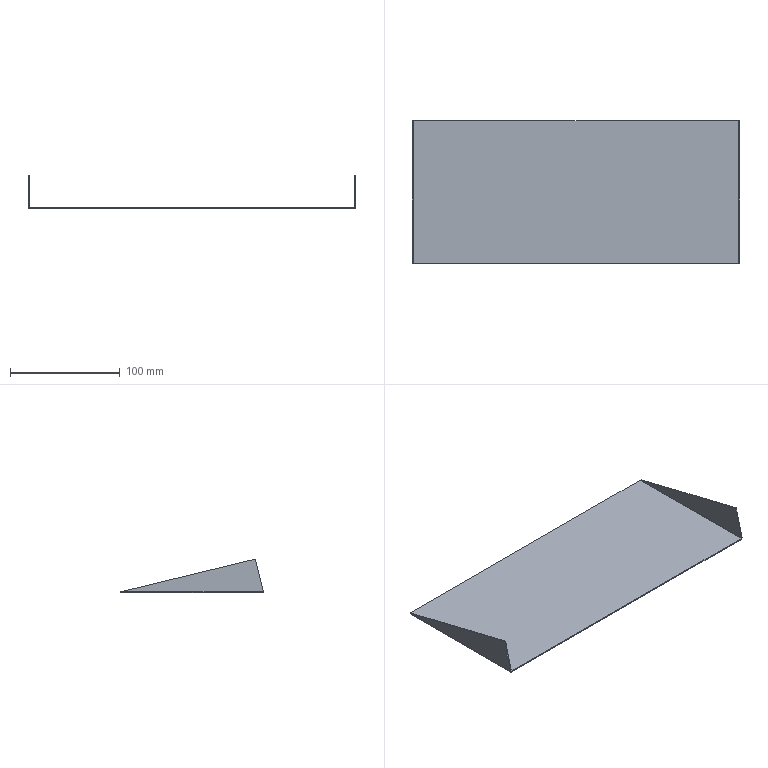Part | SolidWorks | features EdgeFlange 1, FlatPattern 1, MirrorPattern 1, SMBaseFlange 1, SheetMetal 1 | 1 solid | 20 faces | box 299 x 130.5 x 31 mm | volume 42855 mm3 | plane 12 | spline 4 | cylinder 4 | commonest cylinder face diameters 0.4 x2 2.4 x2
STEP:
#1=CARTESIAN_POINT('',(148.3,65.25,-1.));
#2=VERTEX_POINT('',#1);
#3=CARTESIAN_POINT('',(148.3,-65.25,-1.));
#4=VERTEX_POINT('',#3);
#5=CARTESIAN_POINT('',(148.3,65.25,-1.));
#6=DIRECTION('',(0.,-1.,0.));
#7=VECTOR('',#6,1000.);
#8=LINE('',#5,#7);
#9=EDGE_CURVE('',#2,#4,#8,.T.);
#10=ORIENTED_EDGE('',*,*,#9,.T.);
#11=CARTESIAN_POINT('',(-148.3,-65.25,-1.));
#12=VERTEX_POINT('',#11);
#13=CARTESIAN_POINT('',(-149.5,-65.25,-1.));
#14=DIRECTION('',(1.,0.,0.));
#15=VECTOR('',#14,1000.);
#16=LINE('',#13,#15);
#17=EDGE_CURVE('',#12,#4,#16,.T.);
#18=ORIENTED_EDGE('',*,*,#17,.F.);
#19=CARTESIAN_POINT('',(-148.3,65.25,-1.));
#20=VERTEX_POINT('',#19);
#21=CARTESIAN_POINT('',(-148.3,-65.25,-1.));
#22=DIRECTION('',(0.,1.,0.));
#23=VECTOR('',#22,1000.);
#24=LINE('',#21,#23);
#25=EDGE_CURVE('',#12,#20,#24,.T.);
#26=ORIENTED_EDGE('',*,*,#25,.T.);
#27=CARTESIAN_POINT('',(-149.5,65.25,-1.));
#28=DIRECTION('',(-1.,0.,0.));
#29=VECTOR('',#28,1000.);
#30=LINE('',#27,#29);
#31=EDGE_CURVE('',#2,#20,#30,.T.);
#32=ORIENTED_EDGE('',*,*,#31,.F.);
#33=EDGE_LOOP('',(#10,#18,#26,#32));
#34=FACE_OUTER_BOUND('',#33,.T.);
#35=CARTESIAN_POINT('',(0.,0.,-1.));
#36=DIRECTION('',(0.,0.,1.));
#37=DIRECTION('',(1.,0.,0.));
#38=AXIS2_PLACEMENT_3D('',#35,#36,#37);
#39=PLANE('',#38);
#40=ADVANCED_FACE('',(#34),#39,.F.);
#41=CARTESIAN_POINT('',(-148.3,-65.25,0.));
#42=VERTEX_POINT('',#41);
#43=CARTESIAN_POINT('',(148.3,-65.25,0.));
#44=VERTEX_POINT('',#43);
#45=CARTESIAN_POINT('',(-149.5,-65.25,0.));
#46=DIRECTION('',(1.,0.,0.));
#47=VECTOR('',#46,1000.);
#48=LINE('',#45,#47);
#49=EDGE_CURVE('',#42,#44,#48,.T.);
#50=ORIENTED_EDGE('',*,*,#49,.T.);
#51=CARTESIAN_POINT('',(148.3,65.25,0.));
#52=VERTEX_POINT('',#51);
#53=CARTESIAN_POINT('',(148.3,65.25,0.));
#54=DIRECTION('',(0.,-1.,0.));
#55=VECTOR('',#54,1000.);
#56=LINE('',#53,#55);
#57=EDGE_CURVE('',#52,#44,#56,.T.);
#58=ORIENTED_EDGE('',*,*,#57,.F.);
#59=CARTESIAN_POINT('',(-148.3,65.25,0.));
#60=VERTEX_POINT('',#59);
#61=CARTESIAN_POINT('',(-149.5,65.25,0.));
#62=DIRECTION('',(-1.,0.,0.));
#63=VECTOR('',#62,1000.);
#64=LINE('',#61,#63);
#65=EDGE_CURVE('',#52,#60,#64,.T.);
#66=ORIENTED_EDGE('',*,*,#65,.T.);
#67=CARTESIAN_POINT('',(-148.3,-65.25,0.));
#68=DIRECTION('',(0.,1.,0.));
#69=VECTOR('',#68,1000.);
#70=LINE('',#67,#69);
#71=EDGE_CURVE('',#42,#60,#70,.T.);
#72=ORIENTED_EDGE('',*,*,#71,.F.);
#73=EDGE_LOOP('',(#50,#58,#66,#72));
#74=FACE_OUTER_BOUND('',#73,.T.);
#75=CARTESIAN_POINT('',(0.,0.,0.));
#76=DIRECTION('',(0.,0.,1.));
#77=DIRECTION('',(1.,0.,0.));
#78=AXIS2_PLACEMENT_3D('',#75,#76,#77);
#79=PLANE('',#78);
#80=ADVANCED_FACE('',(#74),#79,.T.);
#81=ORIENTED_EDGE('',*,*,#65,.F.);
#82=CARTESIAN_POINT('',(148.3,65.25,0.));
#83=DIRECTION('',(0.,0.,-1.));
#84=VECTOR('',#83,1000.);
#85=LINE('',#82,#84);
#86=EDGE_CURVE('',#52,#2,#85,.T.);
#87=ORIENTED_EDGE('',*,*,#86,.T.);
#88=ORIENTED_EDGE('',*,*,#31,.T.);
#89=CARTESIAN_POINT('',(-148.3,65.25,0.));
#90=DIRECTION('',(0.,0.,-1.));
#91=VECTOR('',#90,1000.);
#92=LINE('',#89,#91);
#93=EDGE_CURVE('',#60,#20,#92,.T.);
#94=ORIENTED_EDGE('',*,*,#93,.F.);
#95=EDGE_LOOP('',(#81,#87,#88,#94));
#96=FACE_OUTER_BOUND('',#95,.T.);
#97=CARTESIAN_POINT('',(-149.5,65.25,-1.));
#98=DIRECTION('',(0.,1.,0.));
#99=DIRECTION('',(0.,0.,1.));
#100=AXIS2_PLACEMENT_3D('',#97,#98,#99);
#101=PLANE('',#100);
#102=ADVANCED_FACE('',(#96),#101,.T.);
#103=CARTESIAN_POINT('',(148.3,-65.25,0.));
#104=DIRECTION('',(0.,0.,-1.));
#105=VECTOR('',#104,1000.);
#106=LINE('',#103,#105);
#107=EDGE_CURVE('',#44,#4,#106,.T.);
#108=ORIENTED_EDGE('',*,*,#107,.F.);
#109=ORIENTED_EDGE('',*,*,#49,.F.);
#110=CARTESIAN_POINT('',(-148.3,-65.25,0.));
#111=DIRECTION('',(0.,0.,-1.));
#112=VECTOR('',#111,1000.);
#113=LINE('',#110,#112);
#114=EDGE_CURVE('',#42,#12,#113,.T.);
#115=ORIENTED_EDGE('',*,*,#114,.T.);
#116=ORIENTED_EDGE('',*,*,#17,.T.);
#117=EDGE_LOOP('',(#108,#109,#115,#116));
#118=FACE_OUTER_BOUND('',#117,.T.);
#119=CARTESIAN_POINT('',(-149.5,-65.25,-1.));
#120=DIRECTION('',(0.,-1.,0.));
#121=DIRECTION('',(0.,0.,-1.));
#122=AXIS2_PLACEMENT_3D('',#119,#120,#121);
#123=PLANE('',#122);
#124=ADVANCED_FACE('',(#118),#123,.T.);
#125=CARTESIAN_POINT('',(-148.5,64.429,0.2));
#126=VERTEX_POINT('',#125);
#127=CARTESIAN_POINT('',(-149.5,64.429,0.2));
#128=VERTEX_POINT('',#127);
#129=CARTESIAN_POINT('',(-149.5,64.429,0.2));
#130=DIRECTION('',(-1.,0.,0.));
#131=VECTOR('',#130,1000.);
#132=LINE('',#129,#131);
#133=EDGE_CURVE('',#126,#128,#132,.T.);
#134=ORIENTED_EDGE('',*,*,#133,.F.);
#135=CARTESIAN_POINT('',(-148.3,65.25,0.));
#136=CARTESIAN_POINT('',(-148.352,65.113,0.));
#137=CARTESIAN_POINT('',(-148.404,64.976,0.02155));
#138=CARTESIAN_POINT('',(-148.478,64.702,0.0956));
#139=CARTESIAN_POINT('',(-148.5,64.566,0.1476));
#140=CARTESIAN_POINT('',(-148.5,64.429,0.2));
#141=B_SPLINE_CURVE_WITH_KNOTS('',3,(#135,#136,#137,#138,#139,#140),.UNSPECIFIED.,.F.,.F.,(4,2,4),(0.,0.5,1.),.UNSPECIFIED.);
#142=EDGE_CURVE('',#60,#126,#141,.T.);
#143=ORIENTED_EDGE('',*,*,#142,.F.);
#144=ORIENTED_EDGE('',*,*,#93,.T.);
#145=CARTESIAN_POINT('',(-148.3,65.25,-1.));
#146=CARTESIAN_POINT('',(-148.459,65.181,-1.));
#147=CARTESIAN_POINT('',(-148.612,65.114,-0.9695));
#148=CARTESIAN_POINT('',(-148.905,64.976,-0.8483));
#149=CARTESIAN_POINT('',(-149.036,64.908,-0.7606));
#150=CARTESIAN_POINT('',(-149.26,64.771,-0.5372));
#151=CARTESIAN_POINT('',(-149.348,64.703,-0.4051));
#152=CARTESIAN_POINT('',(-149.469,64.566,-0.1141));
#153=CARTESIAN_POINT('',(-149.5,64.498,0.04143));
#154=CARTESIAN_POINT('',(-149.5,64.429,0.2));
#155=B_SPLINE_CURVE_WITH_KNOTS('',3,(#145,#146,#147,#148,#149,#150,#151,#152,#153,#154),.UNSPECIFIED.,.F.,.F.,(4,2,2,2,4),(0.,0.0005105,0.001021,0.001532,0.002042),.UNSPECIFIED.);
#156=EDGE_CURVE('',#20,#128,#155,.T.);
#157=ORIENTED_EDGE('',*,*,#156,.T.);
#158=EDGE_LOOP('',(#134,#143,#144,#157));
#159=FACE_OUTER_BOUND('',#158,.T.);
#160=CARTESIAN_POINT('',(-148.3,65.25,-1.01));
#161=CARTESIAN_POINT('',(-148.458,65.182,-1.01));
#162=CARTESIAN_POINT('',(-148.617,65.113,-0.9785));
#163=CARTESIAN_POINT('',(-148.909,64.976,-0.8573));
#164=CARTESIAN_POINT('',(-149.044,64.908,-0.7676));
#165=CARTESIAN_POINT('',(-149.268,64.771,-0.5436));
#166=CARTESIAN_POINT('',(-149.357,64.702,-0.4094));
#167=CARTESIAN_POINT('',(-149.479,64.566,-0.1167));
#168=CARTESIAN_POINT('',(-149.51,64.497,0.04159));
#169=CARTESIAN_POINT('',(-149.51,64.429,0.2));
#170=CARTESIAN_POINT('',(-148.3,65.25,-1.));
#171=CARTESIAN_POINT('',(-148.457,65.182,-1.));
#172=CARTESIAN_POINT('',(-148.614,65.113,-0.9688));
#173=CARTESIAN_POINT('',(-148.904,64.976,-0.8485));
#174=CARTESIAN_POINT('',(-149.037,64.908,-0.7596));
#175=CARTESIAN_POINT('',(-149.26,64.771,-0.5375));
#176=CARTESIAN_POINT('',(-149.349,64.702,-0.4043));
#177=CARTESIAN_POINT('',(-149.469,64.566,-0.1141));
#178=CARTESIAN_POINT('',(-149.5,64.497,0.0429));
#179=CARTESIAN_POINT('',(-149.5,64.429,0.2));
#180=CARTESIAN_POINT('',(-148.3,65.25,0.));
#181=CARTESIAN_POINT('',(-148.326,65.182,0.));
#182=CARTESIAN_POINT('',(-148.352,65.113,0.005205));
#183=CARTESIAN_POINT('',(-148.401,64.976,0.02524));
#184=CARTESIAN_POINT('',(-148.423,64.908,0.04007));
#185=CARTESIAN_POINT('',(-148.46,64.771,0.07709));
#186=CARTESIAN_POINT('',(-148.475,64.702,0.09928));
#187=CARTESIAN_POINT('',(-148.495,64.566,0.1477));
#188=CARTESIAN_POINT('',(-148.5,64.497,0.1738));
#189=CARTESIAN_POINT('',(-148.5,64.429,0.2));
#190=CARTESIAN_POINT('',(-148.3,65.25,0.0101));
#191=CARTESIAN_POINT('',(-148.325,65.182,0.0101));
#192=CARTESIAN_POINT('',(-148.35,65.113,0.01504));
#193=CARTESIAN_POINT('',(-148.396,64.976,0.03407));
#194=CARTESIAN_POINT('',(-148.417,64.908,0.04814));
#195=CARTESIAN_POINT('',(-148.452,64.771,0.0833));
#196=CARTESIAN_POINT('',(-148.466,64.702,0.1044));
#197=CARTESIAN_POINT('',(-148.485,64.566,0.1503));
#198=CARTESIAN_POINT('',(-148.49,64.497,0.1751));
#199=CARTESIAN_POINT('',(-148.49,64.429,0.2));
#200=B_SPLINE_SURFACE_WITH_KNOTS('',1,3,((#160,#161,#162,#163,#164,#165,#166,#167,#168,#169),(#170,#171,#172,#173,#174,#175,#176,#177,#178,#179),(#180,#181,#182,#183,#184,#185,#186,#187,#188,#189),(#190,#191,#192,#193,#194,#195,#196,#197,#198,#199)),.UNSPECIFIED.,.F.,.F.,.F.,(2,1,1,2),(4,2,2,2,4),(-0.01,0.,1.,1.01),(0.,0.25,0.5,0.75,1.),.UNSPECIFIED.);
#201=ADVANCED_FACE('',(#159),#200,.F.);
#202=CARTESIAN_POINT('',(-148.5,-65.201,0.2));
#203=VERTEX_POINT('',#202);
#204=CARTESIAN_POINT('',(-148.5,-65.201,0.2));
#205=CARTESIAN_POINT('',(-148.5,-65.209,0.1476));
#206=CARTESIAN_POINT('',(-148.478,-65.218,0.0956));
#207=CARTESIAN_POINT('',(-148.404,-65.234,0.02155));
#208=CARTESIAN_POINT('',(-148.352,-65.242,0.));
#209=CARTESIAN_POINT('',(-148.3,-65.25,0.));
#210=B_SPLINE_CURVE_WITH_KNOTS('',3,(#204,#205,#206,#207,#208,#209),.UNSPECIFIED.,.F.,.F.,(4,2,4),(0.,0.5,1.),.UNSPECIFIED.);
#211=EDGE_CURVE('',#203,#42,#210,.T.);
#212=ORIENTED_EDGE('',*,*,#211,.F.);
#213=CARTESIAN_POINT('',(-149.5,-65.201,0.2));
#214=VERTEX_POINT('',#213);
#215=CARTESIAN_POINT('',(-148.5,-65.201,0.2));
#216=DIRECTION('',(-1.,0.,0.));
#217=VECTOR('',#216,1000.);
#218=LINE('',#215,#217);
#219=EDGE_CURVE('',#203,#214,#218,.T.);
#220=ORIENTED_EDGE('',*,*,#219,.T.);
#221=CARTESIAN_POINT('',(-149.5,-65.201,0.2));
#222=CARTESIAN_POINT('',(-149.5,-65.205,0.04292));
#223=CARTESIAN_POINT('',(-149.469,-65.209,-0.1141));
#224=CARTESIAN_POINT('',(-149.349,-65.218,-0.4043));
#225=CARTESIAN_POINT('',(-149.26,-65.222,-0.5375));
#226=CARTESIAN_POINT('',(-149.037,-65.23,-0.7596));
#227=CARTESIAN_POINT('',(-148.904,-65.234,-0.8485));
#228=CARTESIAN_POINT('',(-148.614,-65.242,-0.9688));
#229=CARTESIAN_POINT('',(-148.457,-65.246,-1.));
#230=CARTESIAN_POINT('',(-148.3,-65.25,-1.));
#231=B_SPLINE_CURVE_WITH_KNOTS('',3,(#221,#222,#223,#224,#225,#226,#227,#228,#229,#230),.UNSPECIFIED.,.F.,.F.,(4,2,2,2,4),(0.,0.25,0.5,0.75,1.),.UNSPECIFIED.);
#232=EDGE_CURVE('',#214,#12,#231,.T.);
#233=ORIENTED_EDGE('',*,*,#232,.T.);
#234=ORIENTED_EDGE('',*,*,#114,.F.);
#235=EDGE_LOOP('',(#212,#220,#233,#234));
#236=FACE_OUTER_BOUND('',#235,.T.);
#237=CARTESIAN_POINT('',(-149.51,-65.201,0.2));
#238=CARTESIAN_POINT('',(-149.51,-65.205,0.04158));
#239=CARTESIAN_POINT('',(-149.479,-65.209,-0.1167));
#240=CARTESIAN_POINT('',(-149.357,-65.218,-0.4094));
#241=CARTESIAN_POINT('',(-149.268,-65.222,-0.5436));
#242=CARTESIAN_POINT('',(-149.044,-65.23,-0.7676));
#243=CARTESIAN_POINT('',(-148.909,-65.234,-0.8573));
#244=CARTESIAN_POINT('',(-148.617,-65.242,-0.9785));
#245=CARTESIAN_POINT('',(-148.458,-65.246,-1.01));
#246=CARTESIAN_POINT('',(-148.3,-65.25,-1.01));
#247=CARTESIAN_POINT('',(-149.5,-65.201,0.2));
#248=CARTESIAN_POINT('',(-149.5,-65.205,0.04289));
#249=CARTESIAN_POINT('',(-149.469,-65.209,-0.1141));
#250=CARTESIAN_POINT('',(-149.349,-65.218,-0.4043));
#251=CARTESIAN_POINT('',(-149.26,-65.222,-0.5375));
#252=CARTESIAN_POINT('',(-149.037,-65.23,-0.7596));
#253=CARTESIAN_POINT('',(-148.904,-65.234,-0.8485));
#254=CARTESIAN_POINT('',(-148.614,-65.242,-0.9688));
#255=CARTESIAN_POINT('',(-148.457,-65.246,-1.));
#256=CARTESIAN_POINT('',(-148.3,-65.25,-1.));
#257=CARTESIAN_POINT('',(-148.5,-65.201,0.2));
#258=CARTESIAN_POINT('',(-148.5,-65.205,0.1738));
#259=CARTESIAN_POINT('',(-148.495,-65.209,0.1477));
#260=CARTESIAN_POINT('',(-148.475,-65.218,0.09928));
#261=CARTESIAN_POINT('',(-148.46,-65.222,0.07709));
#262=CARTESIAN_POINT('',(-148.423,-65.23,0.04007));
#263=CARTESIAN_POINT('',(-148.401,-65.234,0.02524));
#264=CARTESIAN_POINT('',(-148.352,-65.242,0.005205));
#265=CARTESIAN_POINT('',(-148.326,-65.246,0.));
#266=CARTESIAN_POINT('',(-148.3,-65.25,0.));
#267=CARTESIAN_POINT('',(-148.49,-65.201,0.2));
#268=CARTESIAN_POINT('',(-148.49,-65.205,0.1751));
#269=CARTESIAN_POINT('',(-148.485,-65.209,0.1503));
#270=CARTESIAN_POINT('',(-148.466,-65.218,0.1044));
#271=CARTESIAN_POINT('',(-148.452,-65.222,0.0833));
#272=CARTESIAN_POINT('',(-148.417,-65.23,0.04814));
#273=CARTESIAN_POINT('',(-148.396,-65.234,0.03407));
#274=CARTESIAN_POINT('',(-148.35,-65.242,0.01504));
#275=CARTESIAN_POINT('',(-148.325,-65.246,0.0101));
#276=CARTESIAN_POINT('',(-148.3,-65.25,0.0101));
#277=B_SPLINE_SURFACE_WITH_KNOTS('',1,3,((#237,#238,#239,#240,#241,#242,#243,#244,#245,#246),(#247,#248,#249,#250,#251,#252,#253,#254,#255,#256),(#257,#258,#259,#260,#261,#262,#263,#264,#265,#266),(#267,#268,#269,#270,#271,#272,#273,#274,#275,#276)),.UNSPECIFIED.,.F.,.F.,.F.,(2,1,1,2),(4,2,2,2,4),(-0.01,0.,1.,1.01),(0.,0.25,0.5,0.75,1.),.UNSPECIFIED.);
#278=ADVANCED_FACE('',(#236),#277,.F.);
#279=ORIENTED_EDGE('',*,*,#25,.F.);
#280=ORIENTED_EDGE('',*,*,#232,.F.);
#281=CARTESIAN_POINT('',(-149.5,64.429,0.2));
#282=DIRECTION('',(0.,1.,0.));
#283=VECTOR('',#282,1000.);
#284=LINE('',#281,#283);
#285=EDGE_CURVE('',#214,#128,#284,.T.);
#286=ORIENTED_EDGE('',*,*,#285,.T.);
#287=ORIENTED_EDGE('',*,*,#156,.F.);
#288=EDGE_LOOP('',(#279,#280,#286,#287));
#289=FACE_OUTER_BOUND('',#288,.T.);
#290=CARTESIAN_POINT('',(-148.3,-65.25,0.2));
#291=DIRECTION('',(0.,-1.,0.));
#292=DIRECTION('',(-1.,0.,0.));
#293=AXIS2_PLACEMENT_3D('',#290,#291,#292);
#294=CYLINDRICAL_SURFACE('',#293,1.2);
#295=ADVANCED_FACE('',(#289),#294,.T.);
#296=ORIENTED_EDGE('',*,*,#71,.T.);
#297=ORIENTED_EDGE('',*,*,#142,.T.);
#298=CARTESIAN_POINT('',(-148.5,64.429,0.2));
#299=DIRECTION('',(0.,-1.,0.));
#300=VECTOR('',#299,1000.);
#301=LINE('',#298,#300);
#302=EDGE_CURVE('',#126,#203,#301,.T.);
#303=ORIENTED_EDGE('',*,*,#302,.T.);
#304=ORIENTED_EDGE('',*,*,#211,.T.);
#305=EDGE_LOOP('',(#296,#297,#303,#304));
#306=FACE_OUTER_BOUND('',#305,.T.);
#307=CARTESIAN_POINT('',(-148.3,-65.25,0.2));
#308=DIRECTION('',(0.,-1.,0.));
#309=DIRECTION('',(-1.,0.,0.));
#310=AXIS2_PLACEMENT_3D('',#307,#308,#309);
#311=CYLINDRICAL_SURFACE('',#310,0.2);
#312=ADVANCED_FACE('',(#306),#311,.F.);
#313=ORIENTED_EDGE('',*,*,#133,.T.);
#314=CARTESIAN_POINT('',(-149.5,-57.944,30.));
#315=VERTEX_POINT('',#314);
#316=CARTESIAN_POINT('',(-149.5,3.653,15.));
#317=DIRECTION('',(0.,0.9716,-0.2366));
#318=VECTOR('',#317,1000.);
#319=LINE('',#316,#318);
#320=EDGE_CURVE('',#315,#128,#319,.T.);
#321=ORIENTED_EDGE('',*,*,#320,.F.);
#322=CARTESIAN_POINT('',(-148.5,-57.944,30.));
#323=VERTEX_POINT('',#322);
#324=CARTESIAN_POINT('',(-149.5,-57.944,30.));
#325=DIRECTION('',(1.,0.,0.));
#326=VECTOR('',#325,1000.);
#327=LINE('',#324,#326);
#328=EDGE_CURVE('',#315,#323,#327,.T.);
#329=ORIENTED_EDGE('',*,*,#328,.T.);
#330=CARTESIAN_POINT('',(-148.5,-57.944,30.));
#331=DIRECTION('',(0.,0.9716,-0.2366));
#332=VECTOR('',#331,1000.);
#333=LINE('',#330,#332);
#334=EDGE_CURVE('',#323,#126,#333,.T.);
#335=ORIENTED_EDGE('',*,*,#334,.T.);
#336=EDGE_LOOP('',(#313,#321,#329,#335));
#337=FACE_OUTER_BOUND('',#336,.T.);
#338=CARTESIAN_POINT('',(-149.5,-57.944,30.));
#339=DIRECTION('',(0.,-0.2366,-0.9716));
#340=DIRECTION('',(0.,0.9716,-0.2366));
#341=AXIS2_PLACEMENT_3D('',#338,#339,#340);
#342=PLANE('',#341);
#343=ADVANCED_FACE('',(#337),#342,.F.);
#344=ORIENTED_EDGE('',*,*,#219,.F.);
#345=CARTESIAN_POINT('',(-148.5,-65.25,0.));
#346=DIRECTION('',(0.,0.2366,0.9716));
#347=VECTOR('',#346,1000.);
#348=LINE('',#345,#347);
#349=EDGE_CURVE('',#203,#323,#348,.T.);
#350=ORIENTED_EDGE('',*,*,#349,.T.);
#351=ORIENTED_EDGE('',*,*,#328,.F.);
#352=CARTESIAN_POINT('',(-149.5,-61.597,15.));
#353=DIRECTION('',(0.,0.2366,0.9716));
#354=VECTOR('',#353,1000.);
#355=LINE('',#352,#354);
#356=EDGE_CURVE('',#214,#315,#355,.T.);
#357=ORIENTED_EDGE('',*,*,#356,.F.);
#358=EDGE_LOOP('',(#344,#350,#351,#357));
#359=FACE_OUTER_BOUND('',#358,.T.);
#360=CARTESIAN_POINT('',(-149.5,-65.25,0.));
#361=DIRECTION('',(0.,0.9716,-0.2366));
#362=DIRECTION('',(0.,0.2366,0.9716));
#363=AXIS2_PLACEMENT_3D('',#360,#361,#362);
#364=PLANE('',#363);
#365=ADVANCED_FACE('',(#359),#364,.F.);
#366=ORIENTED_EDGE('',*,*,#285,.F.);
#367=ORIENTED_EDGE('',*,*,#356,.T.);
#368=ORIENTED_EDGE('',*,*,#320,.T.);
#369=EDGE_LOOP('',(#366,#367,#368));
#370=FACE_OUTER_BOUND('',#369,.T.);
#371=CARTESIAN_POINT('',(-149.5,0.,0.));
#372=DIRECTION('',(1.,0.,0.));
#373=DIRECTION('',(0.,0.,-1.));
#374=AXIS2_PLACEMENT_3D('',#371,#372,#373);
#375=PLANE('',#374);
#376=ADVANCED_FACE('',(#370),#375,.F.);
#377=ORIENTED_EDGE('',*,*,#349,.F.);
#378=ORIENTED_EDGE('',*,*,#302,.F.);
#379=ORIENTED_EDGE('',*,*,#334,.F.);
#380=EDGE_LOOP('',(#377,#378,#379));
#381=FACE_OUTER_BOUND('',#380,.T.);
#382=CARTESIAN_POINT('',(-148.5,0.,0.));
#383=DIRECTION('',(1.,0.,0.));
#384=DIRECTION('',(0.,0.,-1.));
#385=AXIS2_PLACEMENT_3D('',#382,#383,#384);
#386=PLANE('',#385);
#387=ADVANCED_FACE('',(#381),#386,.T.);
#388=CARTESIAN_POINT('',(148.5,-65.201,0.2));
#389=VERTEX_POINT('',#388);
#390=CARTESIAN_POINT('',(149.5,-65.201,0.2));
#391=VERTEX_POINT('',#390);
#392=CARTESIAN_POINT('',(149.5,-65.201,0.2));
#393=DIRECTION('',(1.,0.,0.));
#394=VECTOR('',#393,1000.);
#395=LINE('',#392,#394);
#396=EDGE_CURVE('',#389,#391,#395,.T.);
#397=ORIENTED_EDGE('',*,*,#396,.F.);
#398=CARTESIAN_POINT('',(148.3,-65.25,0.));
#399=CARTESIAN_POINT('',(148.352,-65.242,0.));
#400=CARTESIAN_POINT('',(148.404,-65.234,0.02155));
#401=CARTESIAN_POINT('',(148.478,-65.218,0.0956));
#402=CARTESIAN_POINT('',(148.5,-65.209,0.1476));
#403=CARTESIAN_POINT('',(148.5,-65.201,0.2));
#404=B_SPLINE_CURVE_WITH_KNOTS('',3,(#398,#399,#400,#401,#402,#403),.UNSPECIFIED.,.F.,.F.,(4,2,4),(0.,0.5,1.),.UNSPECIFIED.);
#405=EDGE_CURVE('',#44,#389,#404,.T.);
#406=ORIENTED_EDGE('',*,*,#405,.F.);
#407=ORIENTED_EDGE('',*,*,#107,.T.);
#408=CARTESIAN_POINT('',(148.3,-65.25,-1.));
#409=CARTESIAN_POINT('',(148.457,-65.246,-1.));
#410=CARTESIAN_POINT('',(148.614,-65.242,-0.9688));
#411=CARTESIAN_POINT('',(148.904,-65.234,-0.8485));
#412=CARTESIAN_POINT('',(149.037,-65.23,-0.7596));
#413=CARTESIAN_POINT('',(149.26,-65.222,-0.5375));
#414=CARTESIAN_POINT('',(149.349,-65.218,-0.4043));
#415=CARTESIAN_POINT('',(149.469,-65.209,-0.1141));
#416=CARTESIAN_POINT('',(149.5,-65.205,0.04292));
#417=CARTESIAN_POINT('',(149.5,-65.201,0.2));
#418=B_SPLINE_CURVE_WITH_KNOTS('',3,(#408,#409,#410,#411,#412,#413,#414,#415,#416,#417),.UNSPECIFIED.,.F.,.F.,(4,2,2,2,4),(0.,0.25,0.5,0.75,1.),.UNSPECIFIED.);
#419=EDGE_CURVE('',#4,#391,#418,.T.);
#420=ORIENTED_EDGE('',*,*,#419,.T.);
#421=EDGE_LOOP('',(#397,#406,#407,#420));
#422=FACE_OUTER_BOUND('',#421,.T.);
#423=CARTESIAN_POINT('',(148.3,-65.25,-1.01));
#424=CARTESIAN_POINT('',(148.458,-65.246,-1.01));
#425=CARTESIAN_POINT('',(148.617,-65.242,-0.9785));
#426=CARTESIAN_POINT('',(148.909,-65.234,-0.8573));
#427=CARTESIAN_POINT('',(149.044,-65.23,-0.7676));
#428=CARTESIAN_POINT('',(149.268,-65.222,-0.5436));
#429=CARTESIAN_POINT('',(149.357,-65.218,-0.4094));
#430=CARTESIAN_POINT('',(149.479,-65.209,-0.1167));
#431=CARTESIAN_POINT('',(149.51,-65.205,0.04158));
#432=CARTESIAN_POINT('',(149.51,-65.201,0.2));
#433=CARTESIAN_POINT('',(148.3,-65.25,-1.));
#434=CARTESIAN_POINT('',(148.457,-65.246,-1.));
#435=CARTESIAN_POINT('',(148.614,-65.242,-0.9688));
#436=CARTESIAN_POINT('',(148.904,-65.234,-0.8485));
#437=CARTESIAN_POINT('',(149.037,-65.23,-0.7596));
#438=CARTESIAN_POINT('',(149.26,-65.222,-0.5375));
#439=CARTESIAN_POINT('',(149.349,-65.218,-0.4043));
#440=CARTESIAN_POINT('',(149.469,-65.209,-0.1141));
#441=CARTESIAN_POINT('',(149.5,-65.205,0.04289));
#442=CARTESIAN_POINT('',(149.5,-65.201,0.2));
#443=CARTESIAN_POINT('',(148.3,-65.25,0.));
#444=CARTESIAN_POINT('',(148.326,-65.246,0.));
#445=CARTESIAN_POINT('',(148.352,-65.242,0.005205));
#446=CARTESIAN_POINT('',(148.401,-65.234,0.02524));
#447=CARTESIAN_POINT('',(148.423,-65.23,0.04007));
#448=CARTESIAN_POINT('',(148.46,-65.222,0.07709));
#449=CARTESIAN_POINT('',(148.475,-65.218,0.09928));
#450=CARTESIAN_POINT('',(148.495,-65.209,0.1477));
#451=CARTESIAN_POINT('',(148.5,-65.205,0.1738));
#452=CARTESIAN_POINT('',(148.5,-65.201,0.2));
#453=CARTESIAN_POINT('',(148.3,-65.25,0.0101));
#454=CARTESIAN_POINT('',(148.325,-65.246,0.0101));
#455=CARTESIAN_POINT('',(148.35,-65.242,0.01504));
#456=CARTESIAN_POINT('',(148.396,-65.234,0.03407));
#457=CARTESIAN_POINT('',(148.417,-65.23,0.04814));
#458=CARTESIAN_POINT('',(148.452,-65.222,0.0833));
#459=CARTESIAN_POINT('',(148.466,-65.218,0.1044));
#460=CARTESIAN_POINT('',(148.485,-65.209,0.1503));
#461=CARTESIAN_POINT('',(148.49,-65.205,0.1751));
#462=CARTESIAN_POINT('',(148.49,-65.201,0.2));
#463=B_SPLINE_SURFACE_WITH_KNOTS('',1,3,((#423,#424,#425,#426,#427,#428,#429,#430,#431,#432),(#433,#434,#435,#436,#437,#438,#439,#440,#441,#442),(#443,#444,#445,#446,#447,#448,#449,#450,#451,#452),(#453,#454,#455,#456,#457,#458,#459,#460,#461,#462)),.UNSPECIFIED.,.F.,.F.,.F.,(2,1,1,2),(4,2,2,2,4),(-0.01,0.,1.,1.01),(0.,0.25,0.5,0.75,1.),.UNSPECIFIED.);
#464=ADVANCED_FACE('',(#422),#463,.F.);
#465=CARTESIAN_POINT('',(148.5,64.429,0.2));
#466=VERTEX_POINT('',#465);
#467=CARTESIAN_POINT('',(148.5,64.429,0.2));
#468=CARTESIAN_POINT('',(148.5,64.566,0.1476));
#469=CARTESIAN_POINT('',(148.478,64.702,0.0956));
#470=CARTESIAN_POINT('',(148.404,64.976,0.02155));
#471=CARTESIAN_POINT('',(148.352,65.113,0.));
#472=CARTESIAN_POINT('',(148.3,65.25,0.));
#473=B_SPLINE_CURVE_WITH_KNOTS('',3,(#467,#468,#469,#470,#471,#472),.UNSPECIFIED.,.F.,.F.,(4,2,4),(0.,0.5,1.),.UNSPECIFIED.);
#474=EDGE_CURVE('',#466,#52,#473,.T.);
#475=ORIENTED_EDGE('',*,*,#474,.F.);
#476=CARTESIAN_POINT('',(149.5,64.429,0.2));
#477=VERTEX_POINT('',#476);
#478=CARTESIAN_POINT('',(148.5,64.429,0.2));
#479=DIRECTION('',(1.,0.,0.));
#480=VECTOR('',#479,1000.);
#481=LINE('',#478,#480);
#482=EDGE_CURVE('',#466,#477,#481,.T.);
#483=ORIENTED_EDGE('',*,*,#482,.T.);
#484=CARTESIAN_POINT('',(149.5,64.429,0.2));
#485=CARTESIAN_POINT('',(149.5,64.498,0.04143));
#486=CARTESIAN_POINT('',(149.47,64.565,-0.1121));
#487=CARTESIAN_POINT('',(149.348,64.703,-0.4051));
#488=CARTESIAN_POINT('',(149.261,64.77,-0.5364));
#489=CARTESIAN_POINT('',(149.037,64.908,-0.76));
#490=CARTESIAN_POINT('',(148.905,64.976,-0.8482));
#491=CARTESIAN_POINT('',(148.614,65.113,-0.9688));
#492=CARTESIAN_POINT('',(148.459,65.181,-1.));
#493=CARTESIAN_POINT('',(148.3,65.25,-1.));
#494=B_SPLINE_CURVE_WITH_KNOTS('',3,(#484,#485,#486,#487,#488,#489,#490,#491,#492,#493),.UNSPECIFIED.,.F.,.F.,(4,2,2,2,4),(0.,0.0005105,0.001021,0.001532,0.002042),.UNSPECIFIED.);
#495=EDGE_CURVE('',#477,#2,#494,.T.);
#496=ORIENTED_EDGE('',*,*,#495,.T.);
#497=ORIENTED_EDGE('',*,*,#86,.F.);
#498=EDGE_LOOP('',(#475,#483,#496,#497));
#499=FACE_OUTER_BOUND('',#498,.T.);
#500=CARTESIAN_POINT('',(149.51,64.429,0.2));
#501=CARTESIAN_POINT('',(149.51,64.497,0.04159));
#502=CARTESIAN_POINT('',(149.479,64.566,-0.1167));
#503=CARTESIAN_POINT('',(149.357,64.702,-0.4094));
#504=CARTESIAN_POINT('',(149.268,64.771,-0.5436));
#505=CARTESIAN_POINT('',(149.044,64.908,-0.7676));
#506=CARTESIAN_POINT('',(148.909,64.976,-0.8573));
#507=CARTESIAN_POINT('',(148.617,65.113,-0.9785));
#508=CARTESIAN_POINT('',(148.458,65.182,-1.01));
#509=CARTESIAN_POINT('',(148.3,65.25,-1.01));
#510=CARTESIAN_POINT('',(149.5,64.429,0.2));
#511=CARTESIAN_POINT('',(149.5,64.497,0.0429));
#512=CARTESIAN_POINT('',(149.469,64.566,-0.1141));
#513=CARTESIAN_POINT('',(149.349,64.702,-0.4043));
#514=CARTESIAN_POINT('',(149.26,64.771,-0.5375));
#515=CARTESIAN_POINT('',(149.037,64.908,-0.7596));
#516=CARTESIAN_POINT('',(148.904,64.976,-0.8485));
#517=CARTESIAN_POINT('',(148.614,65.113,-0.9688));
#518=CARTESIAN_POINT('',(148.457,65.182,-1.));
#519=CARTESIAN_POINT('',(148.3,65.25,-1.));
#520=CARTESIAN_POINT('',(148.5,64.429,0.2));
#521=CARTESIAN_POINT('',(148.5,64.497,0.1738));
#522=CARTESIAN_POINT('',(148.495,64.566,0.1477));
#523=CARTESIAN_POINT('',(148.475,64.702,0.09928));
#524=CARTESIAN_POINT('',(148.46,64.771,0.07709));
#525=CARTESIAN_POINT('',(148.423,64.908,0.04007));
#526=CARTESIAN_POINT('',(148.401,64.976,0.02524));
#527=CARTESIAN_POINT('',(148.352,65.113,0.005205));
#528=CARTESIAN_POINT('',(148.326,65.182,0.));
#529=CARTESIAN_POINT('',(148.3,65.25,0.));
#530=CARTESIAN_POINT('',(148.49,64.429,0.2));
#531=CARTESIAN_POINT('',(148.49,64.497,0.1751));
#532=CARTESIAN_POINT('',(148.485,64.566,0.1503));
#533=CARTESIAN_POINT('',(148.466,64.702,0.1044));
#534=CARTESIAN_POINT('',(148.452,64.771,0.0833));
#535=CARTESIAN_POINT('',(148.417,64.908,0.04814));
#536=CARTESIAN_POINT('',(148.396,64.976,0.03407));
#537=CARTESIAN_POINT('',(148.35,65.113,0.01504));
#538=CARTESIAN_POINT('',(148.325,65.182,0.0101));
#539=CARTESIAN_POINT('',(148.3,65.25,0.0101));
#540=B_SPLINE_SURFACE_WITH_KNOTS('',1,3,((#500,#501,#502,#503,#504,#505,#506,#507,#508,#509),(#510,#511,#512,#513,#514,#515,#516,#517,#518,#519),(#520,#521,#522,#523,#524,#525,#526,#527,#528,#529),(#530,#531,#532,#533,#534,#535,#536,#537,#538,#539)),.UNSPECIFIED.,.F.,.F.,.F.,(2,1,1,2),(4,2,2,2,4),(-0.01,0.,1.,1.01),(0.,0.25,0.5,0.75,1.),.UNSPECIFIED.);
#541=ADVANCED_FACE('',(#499),#540,.F.);
#542=ORIENTED_EDGE('',*,*,#9,.F.);
#543=ORIENTED_EDGE('',*,*,#495,.F.);
#544=CARTESIAN_POINT('',(149.5,-65.201,0.2));
#545=DIRECTION('',(0.,-1.,0.));
#546=VECTOR('',#545,1000.);
#547=LINE('',#544,#546);
#548=EDGE_CURVE('',#477,#391,#547,.T.);
#549=ORIENTED_EDGE('',*,*,#548,.T.);
#550=ORIENTED_EDGE('',*,*,#419,.F.);
#551=EDGE_LOOP('',(#542,#543,#549,#550));
#552=FACE_OUTER_BOUND('',#551,.T.);
#553=CARTESIAN_POINT('',(148.3,65.25,0.2));
#554=DIRECTION('',(0.,1.,0.));
#555=DIRECTION('',(1.,0.,0.));
#556=AXIS2_PLACEMENT_3D('',#553,#554,#555);
#557=CYLINDRICAL_SURFACE('',#556,1.2);
#558=ADVANCED_FACE('',(#552),#557,.T.);
#559=ORIENTED_EDGE('',*,*,#57,.T.);
#560=ORIENTED_EDGE('',*,*,#405,.T.);
#561=CARTESIAN_POINT('',(148.5,-65.201,0.2));
#562=DIRECTION('',(0.,1.,0.));
#563=VECTOR('',#562,1000.);
#564=LINE('',#561,#563);
#565=EDGE_CURVE('',#389,#466,#564,.T.);
#566=ORIENTED_EDGE('',*,*,#565,.T.);
#567=ORIENTED_EDGE('',*,*,#474,.T.);
#568=EDGE_LOOP('',(#559,#560,#566,#567));
#569=FACE_OUTER_BOUND('',#568,.T.);
#570=CARTESIAN_POINT('',(148.3,65.25,0.2));
#571=DIRECTION('',(0.,1.,0.));
#572=DIRECTION('',(1.,0.,0.));
#573=AXIS2_PLACEMENT_3D('',#570,#571,#572);
#574=CYLINDRICAL_SURFACE('',#573,0.2);
#575=ADVANCED_FACE('',(#569),#574,.F.);
#576=CARTESIAN_POINT('',(149.5,-57.944,30.));
#577=VERTEX_POINT('',#576);
#578=CARTESIAN_POINT('',(149.5,-57.944,30.));
#579=DIRECTION('',(0.,0.9716,-0.2366));
#580=VECTOR('',#579,1000.);
#581=LINE('',#578,#580);
#582=EDGE_CURVE('',#577,#477,#581,.T.);
#583=ORIENTED_EDGE('',*,*,#582,.T.);
#584=ORIENTED_EDGE('',*,*,#482,.F.);
#585=CARTESIAN_POINT('',(148.5,-57.944,30.));
#586=VERTEX_POINT('',#585);
#587=CARTESIAN_POINT('',(148.5,3.653,15.));
#588=DIRECTION('',(0.,0.9716,-0.2366));
#589=VECTOR('',#588,1000.);
#590=LINE('',#587,#589);
#591=EDGE_CURVE('',#586,#466,#590,.T.);
#592=ORIENTED_EDGE('',*,*,#591,.F.);
#593=CARTESIAN_POINT('',(149.5,-57.944,30.));
#594=DIRECTION('',(-1.,0.,0.));
#595=VECTOR('',#594,1000.);
#596=LINE('',#593,#595);
#597=EDGE_CURVE('',#577,#586,#596,.T.);
#598=ORIENTED_EDGE('',*,*,#597,.F.);
#599=EDGE_LOOP('',(#583,#584,#592,#598));
#600=FACE_OUTER_BOUND('',#599,.T.);
#601=CARTESIAN_POINT('',(149.5,-57.944,30.));
#602=DIRECTION('',(0.,0.2366,0.9716));
#603=DIRECTION('',(0.,-0.9716,0.2366));
#604=AXIS2_PLACEMENT_3D('',#601,#602,#603);
#605=PLANE('',#604);
#606=ADVANCED_FACE('',(#600),#605,.T.);
#607=CARTESIAN_POINT('',(148.5,-61.597,15.));
#608=DIRECTION('',(0.,0.2366,0.9716));
#609=VECTOR('',#608,1000.);
#610=LINE('',#607,#609);
#611=EDGE_CURVE('',#389,#586,#610,.T.);
#612=ORIENTED_EDGE('',*,*,#611,.F.);
#613=ORIENTED_EDGE('',*,*,#396,.T.);
#614=CARTESIAN_POINT('',(149.5,-65.25,0.));
#615=DIRECTION('',(0.,0.2366,0.9716));
#616=VECTOR('',#615,1000.);
#617=LINE('',#614,#616);
#618=EDGE_CURVE('',#391,#577,#617,.T.);
#619=ORIENTED_EDGE('',*,*,#618,.T.);
#620=ORIENTED_EDGE('',*,*,#597,.T.);
#621=EDGE_LOOP('',(#612,#613,#619,#620));
#622=FACE_OUTER_BOUND('',#621,.T.);
#623=CARTESIAN_POINT('',(149.5,-65.25,0.));
#624=DIRECTION('',(0.,-0.9716,0.2366));
#625=DIRECTION('',(0.,-0.2366,-0.9716));
#626=AXIS2_PLACEMENT_3D('',#623,#624,#625);
#627=PLANE('',#626);
#628=ADVANCED_FACE('',(#622),#627,.T.);
#629=ORIENTED_EDGE('',*,*,#548,.F.);
#630=ORIENTED_EDGE('',*,*,#582,.F.);
#631=ORIENTED_EDGE('',*,*,#618,.F.);
#632=EDGE_LOOP('',(#629,#630,#631));
#633=FACE_OUTER_BOUND('',#632,.T.);
#634=CARTESIAN_POINT('',(149.5,0.,0.));
#635=DIRECTION('',(-1.,0.,0.));
#636=DIRECTION('',(0.,0.,-1.));
#637=AXIS2_PLACEMENT_3D('',#634,#635,#636);
#638=PLANE('',#637);
#639=ADVANCED_FACE('',(#633),#638,.F.);
#640=ORIENTED_EDGE('',*,*,#591,.T.);
#641=ORIENTED_EDGE('',*,*,#565,.F.);
#642=ORIENTED_EDGE('',*,*,#611,.T.);
#643=EDGE_LOOP('',(#640,#641,#642));
#644=FACE_OUTER_BOUND('',#643,.T.);
#645=CARTESIAN_POINT('',(148.5,0.,0.));
#646=DIRECTION('',(-1.,0.,0.));
#647=DIRECTION('',(0.,0.,-1.));
#648=AXIS2_PLACEMENT_3D('',#645,#646,#647);
#649=PLANE('',#648);
#650=ADVANCED_FACE('',(#644),#649,.T.);
#651=CLOSED_SHELL('',(#40,#80,#102,#124,#201,#278,#295,#312,#343,#365,#376,#387,#464,#541,#558,#575,#606,#628,#639,#650));
#652=MANIFOLD_SOLID_BREP('',#651);
#653=CARTESIAN_POINT('',(0.,0.,0.));
#654=DIRECTION('',(0.,0.,1.));
#655=DIRECTION('',(1.,0.,0.));
#656=AXIS2_PLACEMENT_3D('',#653,#654,#655);
#657=(LENGTH_UNIT()NAMED_UNIT(*)SI_UNIT(.MILLI.,.METRE.));
#658=UNCERTAINTY_MEASURE_WITH_UNIT(LENGTH_MEASURE(0.00001),#657,'','');
#659=(NAMED_UNIT(*)PLANE_ANGLE_UNIT()SI_UNIT($,.RADIAN.));
#660=(NAMED_UNIT(*)SI_UNIT($,.STERADIAN.)SOLID_ANGLE_UNIT());
#661=(GEOMETRIC_REPRESENTATION_CONTEXT(3)GLOBAL_UNCERTAINTY_ASSIGNED_CONTEXT((#658))GLOBAL_UNIT_ASSIGNED_CONTEXT((#657,#659,#660))REPRESENTATION_CONTEXT('',''));
#662=ADVANCED_BREP_SHAPE_REPRESENTATION('',(#652,#656),#661);